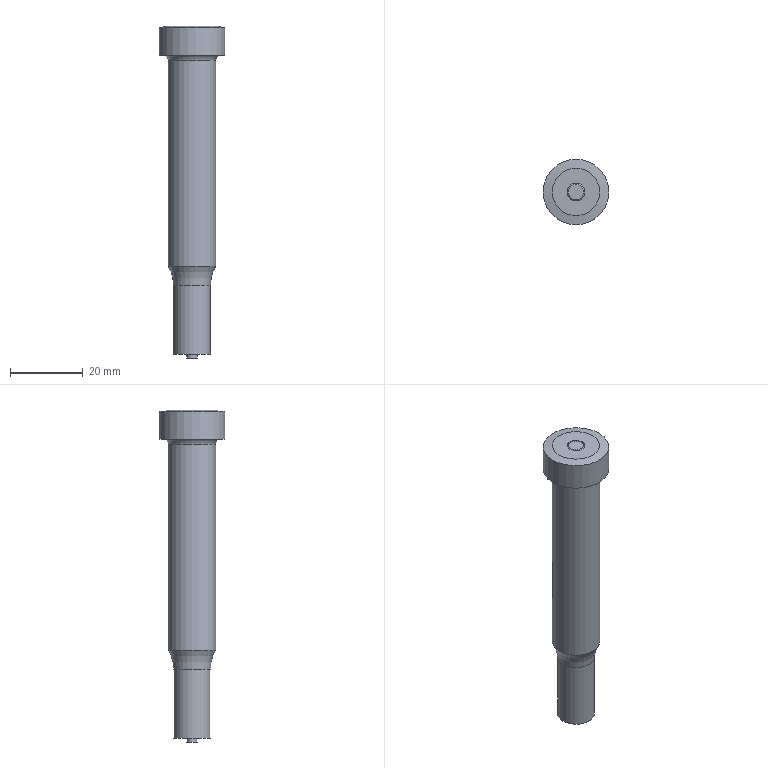Part | STEP file | 1_id2866_x_t | 1 solid | 22 faces | box 18 x 18 x 91 mm | volume 11747 mm3 | cylinder 9 | plane 8 | cone 2 | torus 2 | spline 1 | commonest cylinder face diameters 2.8 x2 4.4 x1 4.401 x1 4.9 x1 4.901 x1 10.15 x1